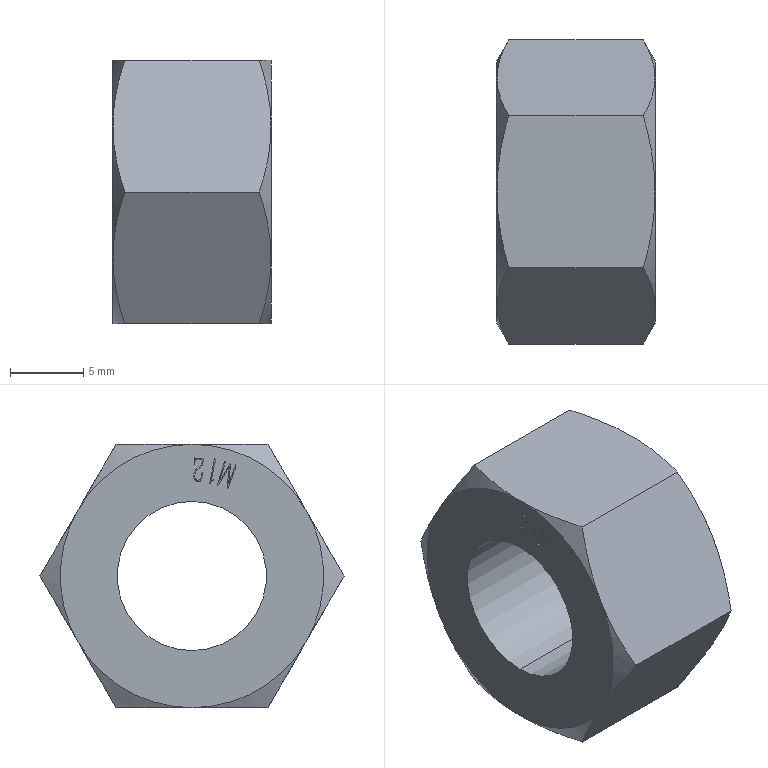Part | SolidWorks | features 3DProfileFeature 1, Extrusion 1, HoleWzd 1, ICE 1, MirrorPattern 1, RevCut 1 | 1 solid | 81 faces | box 10.8 x 20.785 x 18 mm | volume 2135 mm3 | plane 45 | spline 22 | cone 12 | cylinder 2 | commonest cylinder face diameters 10.2 x2